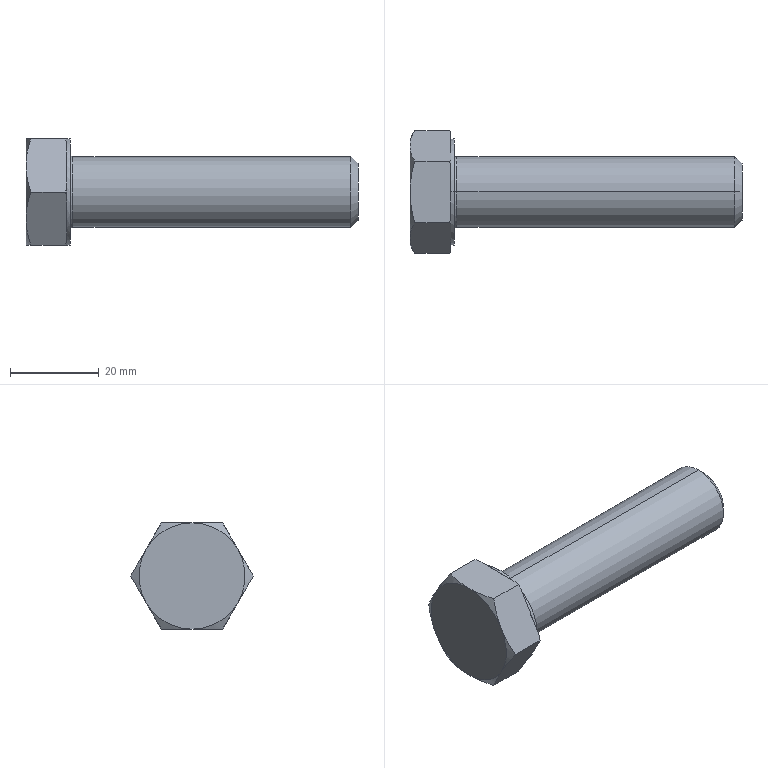Part | SolidWorks | features RevCut 4, Chamfer 1, Extrusion 1, Fillet 1, LPattern 1, Revolution 1 | 1 solid | 35 faces | box 75 x 27.713 x 24 mm | volume 17949 mm3 | plane 15 | cone 14 | cylinder 4 | torus 2 | commonest cylinder face diameters 16 x2 24 x2
STEP:
#1=CARTESIAN_POINT('',(10.6,0.,8.));
#2=VERTEX_POINT('',#1);
#3=CARTESIAN_POINT('',(10.6,0.,-8.));
#4=VERTEX_POINT('',#3);
#5=CARTESIAN_POINT('',(10.6,0.,0.));
#6=DIRECTION('',(1.,0.,0.));
#7=DIRECTION('',(0.,0.,-1.));
#8=AXIS2_PLACEMENT_3D('',#5,#6,#7);
#9=CIRCLE('',#8,8.);
#10=EDGE_CURVE('',#2,#4,#9,.T.);
#11=ORIENTED_EDGE('',*,*,#10,.F.);
#12=CARTESIAN_POINT('',(10.,0.,8.6));
#13=VERTEX_POINT('',#12);
#14=CARTESIAN_POINT('',(10.6,0.,8.6));
#15=DIRECTION('',(0.,1.,0.));
#16=DIRECTION('',(0.,0.,1.));
#17=AXIS2_PLACEMENT_3D('',#14,#15,#16);
#18=CIRCLE('',#17,0.6);
#19=EDGE_CURVE('',#2,#13,#18,.T.);
#20=ORIENTED_EDGE('',*,*,#19,.T.);
#21=CARTESIAN_POINT('',(10.,0.,-8.6));
#22=VERTEX_POINT('',#21);
#23=CARTESIAN_POINT('',(10.,0.,0.));
#24=DIRECTION('',(-1.,0.,0.));
#25=DIRECTION('',(0.,0.,-1.));
#26=AXIS2_PLACEMENT_3D('',#23,#24,#25);
#27=CIRCLE('',#26,8.6);
#28=EDGE_CURVE('',#22,#13,#27,.T.);
#29=ORIENTED_EDGE('',*,*,#28,.F.);
#30=CARTESIAN_POINT('',(10.6,0.,-8.6));
#31=DIRECTION('',(0.,-1.,0.));
#32=DIRECTION('',(0.,0.,-1.));
#33=AXIS2_PLACEMENT_3D('',#30,#31,#32);
#34=CIRCLE('',#33,0.6);
#35=EDGE_CURVE('',#4,#22,#34,.T.);
#36=ORIENTED_EDGE('',*,*,#35,.F.);
#37=EDGE_LOOP('',(#11,#20,#29,#36));
#38=FACE_OUTER_BOUND('',#37,.T.);
#39=CARTESIAN_POINT('',(10.6,0.,0.));
#40=DIRECTION('',(1.,0.,0.));
#41=DIRECTION('',(0.,0.,-1.));
#42=AXIS2_PLACEMENT_3D('',#39,#40,#41);
#43=TOROIDAL_SURFACE('',#42,8.6,0.6);
#44=ADVANCED_FACE('',(#38),#43,.F.);
#45=CARTESIAN_POINT('',(75.,0.,-6.4));
#46=VERTEX_POINT('',#45);
#47=CARTESIAN_POINT('',(75.,0.,6.4));
#48=VERTEX_POINT('',#47);
#49=CARTESIAN_POINT('',(75.,0.,0.));
#50=DIRECTION('',(1.,0.,0.));
#51=DIRECTION('',(0.,0.,1.));
#52=AXIS2_PLACEMENT_3D('',#49,#50,#51);
#53=CIRCLE('',#52,6.4);
#54=EDGE_CURVE('',#46,#48,#53,.T.);
#55=ORIENTED_EDGE('',*,*,#54,.F.);
#56=CARTESIAN_POINT('',(73.4,0.,-8.));
#57=VERTEX_POINT('',#56);
#58=CARTESIAN_POINT('',(73.4,0.,-8.));
#59=DIRECTION('',(-0.7071,0.,-0.7071));
#60=VECTOR('',#59,1000.);
#61=LINE('',#58,#60);
#62=EDGE_CURVE('',#46,#57,#61,.T.);
#63=ORIENTED_EDGE('',*,*,#62,.T.);
#64=CARTESIAN_POINT('',(73.4,0.,8.));
#65=VERTEX_POINT('',#64);
#66=CARTESIAN_POINT('',(73.4,0.,0.));
#67=DIRECTION('',(-1.,0.,0.));
#68=DIRECTION('',(0.,0.,1.));
#69=AXIS2_PLACEMENT_3D('',#66,#67,#68);
#70=CIRCLE('',#69,8.);
#71=EDGE_CURVE('',#65,#57,#70,.T.);
#72=ORIENTED_EDGE('',*,*,#71,.F.);
#73=CARTESIAN_POINT('',(73.4,0.,8.));
#74=DIRECTION('',(-0.7071,0.,0.7071));
#75=VECTOR('',#74,1000.);
#76=LINE('',#73,#75);
#77=EDGE_CURVE('',#48,#65,#76,.T.);
#78=ORIENTED_EDGE('',*,*,#77,.F.);
#79=EDGE_LOOP('',(#55,#63,#72,#78));
#80=FACE_OUTER_BOUND('',#79,.T.);
#81=CARTESIAN_POINT('',(73.4,0.,0.));
#82=DIRECTION('',(-1.,0.,0.));
#83=DIRECTION('',(0.,0.,1.));
#84=AXIS2_PLACEMENT_3D('',#81,#82,#83);
#85=CONICAL_SURFACE('',#84,8.,0.7854);
#86=ADVANCED_FACE('',(#80),#85,.T.);
#87=ORIENTED_EDGE('',*,*,#71,.T.);
#88=CARTESIAN_POINT('',(0.,0.,-8.));
#89=DIRECTION('',(-1.,0.,0.));
#90=VECTOR('',#89,1000.);
#91=LINE('',#88,#90);
#92=EDGE_CURVE('',#57,#4,#91,.T.);
#93=ORIENTED_EDGE('',*,*,#92,.T.);
#94=CARTESIAN_POINT('',(10.6,0.,0.));
#95=DIRECTION('',(1.,0.,0.));
#96=DIRECTION('',(0.,0.,-1.));
#97=AXIS2_PLACEMENT_3D('',#94,#95,#96);
#98=CIRCLE('',#97,8.);
#99=EDGE_CURVE('',#4,#2,#98,.T.);
#100=ORIENTED_EDGE('',*,*,#99,.T.);
#101=CARTESIAN_POINT('',(0.,0.,8.));
#102=DIRECTION('',(-1.,0.,0.));
#103=VECTOR('',#102,1000.);
#104=LINE('',#101,#103);
#105=EDGE_CURVE('',#65,#2,#104,.T.);
#106=ORIENTED_EDGE('',*,*,#105,.F.);
#107=EDGE_LOOP('',(#87,#93,#100,#106));
#108=FACE_OUTER_BOUND('',#107,.T.);
#109=CARTESIAN_POINT('',(0.,0.,0.));
#110=DIRECTION('',(-1.,0.,0.));
#111=DIRECTION('',(0.,0.,1.));
#112=AXIS2_PLACEMENT_3D('',#109,#110,#111);
#113=CYLINDRICAL_SURFACE('',#112,8.);
#114=ADVANCED_FACE('',(#108),#113,.T.);
#115=CARTESIAN_POINT('',(10.,0.,-12.));
#116=VERTEX_POINT('',#115);
#117=CARTESIAN_POINT('',(10.,0.,12.));
#118=VERTEX_POINT('',#117);
#119=CARTESIAN_POINT('',(10.,0.,0.));
#120=DIRECTION('',(1.,0.,0.));
#121=DIRECTION('',(0.,0.,-1.));
#122=AXIS2_PLACEMENT_3D('',#119,#120,#121);
#123=CIRCLE('',#122,12.);
#124=EDGE_CURVE('',#116,#118,#123,.T.);
#125=ORIENTED_EDGE('',*,*,#124,.F.);
#126=CARTESIAN_POINT('',(9.2,0.,-12.));
#127=VERTEX_POINT('',#126);
#128=CARTESIAN_POINT('',(0.,0.,-12.));
#129=DIRECTION('',(-1.,0.,0.));
#130=VECTOR('',#129,1000.);
#131=LINE('',#128,#130);
#132=EDGE_CURVE('',#116,#127,#131,.T.);
#133=ORIENTED_EDGE('',*,*,#132,.T.);
#134=CARTESIAN_POINT('',(9.2,10.392,-6.));
#135=VERTEX_POINT('',#134);
#136=CARTESIAN_POINT('',(9.2,0.,0.));
#137=DIRECTION('',(-1.,0.,0.));
#138=DIRECTION('',(0.,0.,1.));
#139=AXIS2_PLACEMENT_3D('',#136,#137,#138);
#140=CIRCLE('',#139,12.);
#141=EDGE_CURVE('',#135,#127,#140,.T.);
#142=ORIENTED_EDGE('',*,*,#141,.F.);
#143=CARTESIAN_POINT('',(9.2,10.392,6.));
#144=VERTEX_POINT('',#143);
#145=CARTESIAN_POINT('',(9.2,0.,0.));
#146=DIRECTION('',(-1.,0.,0.));
#147=DIRECTION('',(0.,0.,1.));
#148=AXIS2_PLACEMENT_3D('',#145,#146,#147);
#149=CIRCLE('',#148,12.);
#150=EDGE_CURVE('',#144,#135,#149,.T.);
#151=ORIENTED_EDGE('',*,*,#150,.F.);
#152=CARTESIAN_POINT('',(9.2,0.,12.));
#153=VERTEX_POINT('',#152);
#154=CARTESIAN_POINT('',(9.2,0.,0.));
#155=DIRECTION('',(-1.,0.,0.));
#156=DIRECTION('',(0.,0.,1.));
#157=AXIS2_PLACEMENT_3D('',#154,#155,#156);
#158=CIRCLE('',#157,12.);
#159=EDGE_CURVE('',#153,#144,#158,.T.);
#160=ORIENTED_EDGE('',*,*,#159,.F.);
#161=CARTESIAN_POINT('',(0.,0.,12.));
#162=DIRECTION('',(-1.,0.,0.));
#163=VECTOR('',#162,1000.);
#164=LINE('',#161,#163);
#165=EDGE_CURVE('',#118,#153,#164,.T.);
#166=ORIENTED_EDGE('',*,*,#165,.F.);
#167=EDGE_LOOP('',(#125,#133,#142,#151,#160,#166));
#168=FACE_OUTER_BOUND('',#167,.T.);
#169=CARTESIAN_POINT('',(0.,0.,0.));
#170=DIRECTION('',(-1.,0.,0.));
#171=DIRECTION('',(0.,0.,1.));
#172=AXIS2_PLACEMENT_3D('',#169,#170,#171);
#173=CYLINDRICAL_SURFACE('',#172,12.);
#174=ADVANCED_FACE('',(#168),#173,.T.);
#175=CARTESIAN_POINT('',(9.2,7.427,-11.136));
#176=VERTEX_POINT('',#175);
#177=CARTESIAN_POINT('',(9.2,6.928,-12.));
#178=DIRECTION('',(0.,0.5,0.866));
#179=VECTOR('',#178,1000.);
#180=LINE('',#177,#179);
#181=EDGE_CURVE('',#176,#135,#180,.T.);
#182=ORIENTED_EDGE('',*,*,#181,.F.);
#183=CARTESIAN_POINT('',(8.928,6.928,-12.));
#184=VERTEX_POINT('',#183);
#185=CARTESIAN_POINT('',(8.928,6.928,-12.));
#186=CARTESIAN_POINT('',(9.024,7.094,-11.713));
#187=CARTESIAN_POINT('',(9.115,7.26,-11.425));
#188=CARTESIAN_POINT('',(9.2,7.427,-11.136));
#189=B_SPLINE_CURVE_WITH_KNOTS('',3,(#185,#186,#187,#188),.UNSPECIFIED.,.F.,.F.,(4,4),(0.000000238,0.001026),.UNSPECIFIED.);
#190=EDGE_CURVE('',#184,#176,#189,.T.);
#191=ORIENTED_EDGE('',*,*,#190,.F.);
#192=CARTESIAN_POINT('',(1.072,6.928,-12.));
#193=VERTEX_POINT('',#192);
#194=CARTESIAN_POINT('',(10.,6.928,-12.));
#195=DIRECTION('',(-1.,0.,0.));
#196=VECTOR('',#195,1000.);
#197=LINE('',#194,#196);
#198=EDGE_CURVE('',#184,#193,#197,.T.);
#199=ORIENTED_EDGE('',*,*,#198,.T.);
#200=CARTESIAN_POINT('',(0.,10.392,-6.));
#201=VERTEX_POINT('',#200);
#202=CARTESIAN_POINT('',(0.,10.392,-6.));
#203=CARTESIAN_POINT('',(0.,10.098,-6.509));
#204=CARTESIAN_POINT('',(0.02533,9.803,-7.021));
#205=CARTESIAN_POINT('',(0.1234,9.219,-8.033));
#206=CARTESIAN_POINT('',(0.196,8.929,-8.535));
#207=CARTESIAN_POINT('',(0.476,8.063,-10.034));
#208=CARTESIAN_POINT('',(0.7454,7.493,-11.021));
#209=CARTESIAN_POINT('',(1.072,6.928,-12.));
#210=B_SPLINE_CURVE_WITH_KNOTS('',3,(#202,#203,#204,#205,#206,#207,#208,#209),.UNSPECIFIED.,.F.,.F.,(4,2,2,4),(0.00701,0.008756,0.0105,0.01399),.UNSPECIFIED.);
#211=EDGE_CURVE('',#201,#193,#210,.T.);
#212=ORIENTED_EDGE('',*,*,#211,.F.);
#213=CARTESIAN_POINT('',(1.072,13.856,0.));
#214=VERTEX_POINT('',#213);
#215=CARTESIAN_POINT('',(1.072,13.856,0.));
#216=CARTESIAN_POINT('',(0.7446,13.29,-0.9815));
#217=CARTESIAN_POINT('',(0.4751,12.719,-1.97));
#218=CARTESIAN_POINT('',(0.1021,11.565,-3.968));
#219=CARTESIAN_POINT('',(0.,10.982,-4.978));
#220=CARTESIAN_POINT('',(0.,10.392,-6.));
#221=B_SPLINE_CURVE_WITH_KNOTS('',3,(#215,#216,#217,#218,#219,#220),.UNSPECIFIED.,.F.,.F.,(4,2,4),(0.000000238,0.003505,0.00701),.UNSPECIFIED.);
#222=EDGE_CURVE('',#214,#201,#221,.T.);
#223=ORIENTED_EDGE('',*,*,#222,.F.);
#224=CARTESIAN_POINT('',(8.928,13.856,0.));
#225=VERTEX_POINT('',#224);
#226=CARTESIAN_POINT('',(10.,13.856,0.));
#227=DIRECTION('',(-1.,0.,0.));
#228=VECTOR('',#227,1000.);
#229=LINE('',#226,#228);
#230=EDGE_CURVE('',#225,#214,#229,.T.);
#231=ORIENTED_EDGE('',*,*,#230,.F.);
#232=CARTESIAN_POINT('',(9.2,13.358,-0.8637));
#233=VERTEX_POINT('',#232);
#234=CARTESIAN_POINT('',(9.2,13.358,-0.8637));
#235=CARTESIAN_POINT('',(9.115,13.524,-0.575));
#236=CARTESIAN_POINT('',(9.024,13.691,-0.2872));
#237=CARTESIAN_POINT('',(8.928,13.856,0.));
#238=B_SPLINE_CURVE_WITH_KNOTS('',3,(#234,#235,#236,#237),.UNSPECIFIED.,.F.,.F.,(4,4),(0.01297,0.01399),.UNSPECIFIED.);
#239=EDGE_CURVE('',#233,#225,#238,.T.);
#240=ORIENTED_EDGE('',*,*,#239,.F.);
#241=CARTESIAN_POINT('',(9.2,6.928,-12.));
#242=DIRECTION('',(0.,0.5,0.866));
#243=VECTOR('',#242,1000.);
#244=LINE('',#241,#243);
#245=EDGE_CURVE('',#135,#233,#244,.T.);
#246=ORIENTED_EDGE('',*,*,#245,.F.);
#247=EDGE_LOOP('',(#182,#191,#199,#212,#223,#231,#240,#246));
#248=FACE_OUTER_BOUND('',#247,.T.);
#249=CARTESIAN_POINT('',(10.,6.928,-12.));
#250=DIRECTION('',(0.,-0.866,0.5));
#251=DIRECTION('',(0.,-0.5,-0.866));
#252=AXIS2_PLACEMENT_3D('',#249,#250,#251);
#253=PLANE('',#252);
#254=ADVANCED_FACE('',(#248),#253,.F.);
#255=CARTESIAN_POINT('',(9.2,13.358,0.8637));
#256=VERTEX_POINT('',#255);
#257=CARTESIAN_POINT('',(9.2,13.856,0.));
#258=DIRECTION('',(0.,-0.5,0.866));
#259=VECTOR('',#258,1000.);
#260=LINE('',#257,#259);
#261=EDGE_CURVE('',#256,#144,#260,.T.);
#262=ORIENTED_EDGE('',*,*,#261,.F.);
#263=CARTESIAN_POINT('',(8.928,13.856,0.));
#264=CARTESIAN_POINT('',(9.024,13.691,0.2873));
#265=CARTESIAN_POINT('',(9.115,13.524,0.5751));
#266=CARTESIAN_POINT('',(9.2,13.358,0.8637));
#267=B_SPLINE_CURVE_WITH_KNOTS('',3,(#263,#264,#265,#266),.UNSPECIFIED.,.F.,.F.,(4,4),(0.000000238,0.001026),.UNSPECIFIED.);
#268=EDGE_CURVE('',#225,#256,#267,.T.);
#269=ORIENTED_EDGE('',*,*,#268,.F.);
#270=ORIENTED_EDGE('',*,*,#230,.T.);
#271=CARTESIAN_POINT('',(0.,10.392,6.));
#272=VERTEX_POINT('',#271);
#273=CARTESIAN_POINT('',(0.,10.392,6.));
#274=CARTESIAN_POINT('',(0.,10.686,5.491));
#275=CARTESIAN_POINT('',(0.02533,10.982,4.979));
#276=CARTESIAN_POINT('',(0.1234,11.566,3.967));
#277=CARTESIAN_POINT('',(0.196,11.856,3.465));
#278=CARTESIAN_POINT('',(0.476,12.721,1.966));
#279=CARTESIAN_POINT('',(0.7454,13.291,0.9791));
#280=CARTESIAN_POINT('',(1.072,13.856,0.));
#281=B_SPLINE_CURVE_WITH_KNOTS('',3,(#273,#274,#275,#276,#277,#278,#279,#280),.UNSPECIFIED.,.F.,.F.,(4,2,2,4),(0.00701,0.008756,0.0105,0.01399),.UNSPECIFIED.);
#282=EDGE_CURVE('',#272,#214,#281,.T.);
#283=ORIENTED_EDGE('',*,*,#282,.F.);
#284=CARTESIAN_POINT('',(1.072,6.928,12.));
#285=VERTEX_POINT('',#284);
#286=CARTESIAN_POINT('',(1.072,6.928,12.));
#287=CARTESIAN_POINT('',(0.7446,7.495,11.018));
#288=CARTESIAN_POINT('',(0.4751,8.066,10.03));
#289=CARTESIAN_POINT('',(0.1021,9.219,8.032));
#290=CARTESIAN_POINT('',(0.,9.802,7.022));
#291=CARTESIAN_POINT('',(0.,10.392,6.));
#292=B_SPLINE_CURVE_WITH_KNOTS('',3,(#286,#287,#288,#289,#290,#291),.UNSPECIFIED.,.F.,.F.,(4,2,4),(0.000000238,0.003505,0.00701),.UNSPECIFIED.);
#293=EDGE_CURVE('',#285,#272,#292,.T.);
#294=ORIENTED_EDGE('',*,*,#293,.F.);
#295=CARTESIAN_POINT('',(8.928,6.928,12.));
#296=VERTEX_POINT('',#295);
#297=CARTESIAN_POINT('',(10.,6.928,12.));
#298=DIRECTION('',(-1.,0.,0.));
#299=VECTOR('',#298,1000.);
#300=LINE('',#297,#299);
#301=EDGE_CURVE('',#296,#285,#300,.T.);
#302=ORIENTED_EDGE('',*,*,#301,.F.);
#303=CARTESIAN_POINT('',(9.2,7.427,11.136));
#304=VERTEX_POINT('',#303);
#305=CARTESIAN_POINT('',(9.2,7.427,11.136));
#306=CARTESIAN_POINT('',(9.115,7.26,11.425));
#307=CARTESIAN_POINT('',(9.024,7.094,11.713));
#308=CARTESIAN_POINT('',(8.928,6.928,12.));
#309=B_SPLINE_CURVE_WITH_KNOTS('',3,(#305,#306,#307,#308),.UNSPECIFIED.,.F.,.F.,(4,4),(0.01297,0.01399),.UNSPECIFIED.);
#310=EDGE_CURVE('',#304,#296,#309,.T.);
#311=ORIENTED_EDGE('',*,*,#310,.F.);
#312=CARTESIAN_POINT('',(9.2,13.856,0.));
#313=DIRECTION('',(0.,-0.5,0.866));
#314=VECTOR('',#313,1000.);
#315=LINE('',#312,#314);
#316=EDGE_CURVE('',#144,#304,#315,.T.);
#317=ORIENTED_EDGE('',*,*,#316,.F.);
#318=EDGE_LOOP('',(#262,#269,#270,#283,#294,#302,#311,#317));
#319=FACE_OUTER_BOUND('',#318,.T.);
#320=CARTESIAN_POINT('',(10.,13.856,0.));
#321=DIRECTION('',(0.,-0.866,-0.5));
#322=DIRECTION('',(0.,0.5,-0.866));
#323=AXIS2_PLACEMENT_3D('',#320,#321,#322);
#324=PLANE('',#323);
#325=ADVANCED_FACE('',(#319),#324,.F.);
#326=CARTESIAN_POINT('',(9.2,5.931,12.));
#327=VERTEX_POINT('',#326);
#328=CARTESIAN_POINT('',(9.2,6.928,12.));
#329=DIRECTION('',(0.,-1.,0.));
#330=VECTOR('',#329,1000.);
#331=LINE('',#328,#330);
#332=EDGE_CURVE('',#327,#153,#331,.T.);
#333=ORIENTED_EDGE('',*,*,#332,.F.);
#334=CARTESIAN_POINT('',(8.928,6.928,12.));
#335=CARTESIAN_POINT('',(9.024,6.597,12.));
#336=CARTESIAN_POINT('',(9.115,6.265,12.));
#337=CARTESIAN_POINT('',(9.2,5.931,12.));
#338=B_SPLINE_CURVE_WITH_KNOTS('',3,(#334,#335,#336,#337),.UNSPECIFIED.,.F.,.F.,(4,4),(0.03236,0.0334),.UNSPECIFIED.);
#339=EDGE_CURVE('',#296,#327,#338,.T.);
#340=ORIENTED_EDGE('',*,*,#339,.F.);
#341=ORIENTED_EDGE('',*,*,#301,.T.);
#342=CARTESIAN_POINT('',(0.,0.,12.));
#343=VERTEX_POINT('',#342);
#344=CARTESIAN_POINT('',(0.,0.,12.));
#345=CARTESIAN_POINT('',(0.,0.5865,12.));
#346=CARTESIAN_POINT('',(0.02506,1.176,12.));
#347=CARTESIAN_POINT('',(0.1242,2.355,12.));
#348=CARTESIAN_POINT('',(0.1975,2.939,12.));
#349=CARTESIAN_POINT('',(0.4791,4.673,12.));
#350=CARTESIAN_POINT('',(0.7483,5.808,12.));
#351=CARTESIAN_POINT('',(1.072,6.928,12.));
#352=B_SPLINE_CURVE_WITH_KNOTS('',3,(#344,#345,#346,#347,#348,#349,#350,#351),.UNSPECIFIED.,.F.,.F.,(4,2,2,4),(0.01982,0.02158,0.02333,0.02684),.UNSPECIFIED.);
#353=EDGE_CURVE('',#343,#285,#352,.T.);
#354=ORIENTED_EDGE('',*,*,#353,.F.);
#355=CARTESIAN_POINT('',(1.072,-6.928,12.));
#356=VERTEX_POINT('',#355);
#357=CARTESIAN_POINT('',(1.072,-6.928,12.));
#358=CARTESIAN_POINT('',(0.7461,-5.8,12.));
#359=CARTESIAN_POINT('',(0.4736,-4.647,12.));
#360=CARTESIAN_POINT('',(0.1008,-2.335,12.));
#361=CARTESIAN_POINT('',(0.,-1.172,12.));
#362=CARTESIAN_POINT('',(0.,0.,12.));
#363=B_SPLINE_CURVE_WITH_KNOTS('',3,(#357,#358,#359,#360,#361,#362),.UNSPECIFIED.,.F.,.F.,(4,2,4),(0.01281,0.01632,0.01982),.UNSPECIFIED.);
#364=EDGE_CURVE('',#356,#343,#363,.T.);
#365=ORIENTED_EDGE('',*,*,#364,.F.);
#366=CARTESIAN_POINT('',(8.928,-6.928,12.));
#367=VERTEX_POINT('',#366);
#368=CARTESIAN_POINT('',(10.,-6.928,12.));
#369=DIRECTION('',(-1.,0.,0.));
#370=VECTOR('',#369,1000.);
#371=LINE('',#368,#370);
#372=EDGE_CURVE('',#367,#356,#371,.T.);
#373=ORIENTED_EDGE('',*,*,#372,.F.);
#374=CARTESIAN_POINT('',(9.2,-5.931,12.));
#375=VERTEX_POINT('',#374);
#376=CARTESIAN_POINT('',(9.2,-5.931,12.));
#377=CARTESIAN_POINT('',(9.114,-6.265,12.));
#378=CARTESIAN_POINT('',(9.024,-6.598,12.));
#379=CARTESIAN_POINT('',(8.928,-6.928,12.));
#380=B_SPLINE_CURVE_WITH_KNOTS('',3,(#376,#377,#378,#379),.UNSPECIFIED.,.F.,.F.,(4,4),(0.04537,0.0464),.UNSPECIFIED.);
#381=EDGE_CURVE('',#375,#367,#380,.T.);
#382=ORIENTED_EDGE('',*,*,#381,.F.);
#383=CARTESIAN_POINT('',(9.2,6.928,12.));
#384=DIRECTION('',(0.,-1.,0.));
#385=VECTOR('',#384,1000.);
#386=LINE('',#383,#385);
#387=EDGE_CURVE('',#153,#375,#386,.T.);
#388=ORIENTED_EDGE('',*,*,#387,.F.);
#389=EDGE_LOOP('',(#333,#340,#341,#354,#365,#373,#382,#388));
#390=FACE_OUTER_BOUND('',#389,.T.);
#391=CARTESIAN_POINT('',(10.,6.928,12.));
#392=DIRECTION('',(0.,0.,-1.));
#393=DIRECTION('',(0.,1.,0.));
#394=AXIS2_PLACEMENT_3D('',#391,#392,#393);
#395=PLANE('',#394);
#396=ADVANCED_FACE('',(#390),#395,.F.);
#397=CARTESIAN_POINT('',(9.2,-7.427,11.136));
#398=VERTEX_POINT('',#397);
#399=CARTESIAN_POINT('',(9.2,-10.392,6.));
#400=VERTEX_POINT('',#399);
#401=CARTESIAN_POINT('',(9.2,-13.856,0.));
#402=DIRECTION('',(0.,-0.5,-0.866));
#403=VECTOR('',#402,1000.);
#404=LINE('',#401,#403);
#405=EDGE_CURVE('',#398,#400,#404,.T.);
#406=ORIENTED_EDGE('',*,*,#405,.F.);
#407=CARTESIAN_POINT('',(8.928,-6.928,12.));
#408=CARTESIAN_POINT('',(9.024,-7.094,11.713));
#409=CARTESIAN_POINT('',(9.115,-7.26,11.425));
#410=CARTESIAN_POINT('',(9.2,-7.427,11.136));
#411=B_SPLINE_CURVE_WITH_KNOTS('',3,(#407,#408,#409,#410),.UNSPECIFIED.,.F.,.F.,(4,4),(0.000000238,0.001026),.UNSPECIFIED.);
#412=EDGE_CURVE('',#367,#398,#411,.T.);
#413=ORIENTED_EDGE('',*,*,#412,.F.);
#414=ORIENTED_EDGE('',*,*,#372,.T.);
#415=CARTESIAN_POINT('',(0.,-10.392,6.));
#416=VERTEX_POINT('',#415);
#417=CARTESIAN_POINT('',(0.,-10.392,6.));
#418=CARTESIAN_POINT('',(0.,-10.098,6.509));
#419=CARTESIAN_POINT('',(0.02533,-9.803,7.021));
#420=CARTESIAN_POINT('',(0.1234,-9.219,8.033));
#421=CARTESIAN_POINT('',(0.196,-8.929,8.535));
#422=CARTESIAN_POINT('',(0.476,-8.063,10.034));
#423=CARTESIAN_POINT('',(0.7454,-7.493,11.021));
#424=CARTESIAN_POINT('',(1.072,-6.928,12.));
#425=B_SPLINE_CURVE_WITH_KNOTS('',3,(#417,#418,#419,#420,#421,#422,#423,#424),.UNSPECIFIED.,.F.,.F.,(4,2,2,4),(0.00701,0.008756,0.0105,0.01399),.UNSPECIFIED.);
#426=EDGE_CURVE('',#416,#356,#425,.T.);
#427=ORIENTED_EDGE('',*,*,#426,.F.);
#428=CARTESIAN_POINT('',(1.072,-13.856,0.));
#429=VERTEX_POINT('',#428);
#430=CARTESIAN_POINT('',(1.072,-13.856,0.));
#431=CARTESIAN_POINT('',(0.7446,-13.29,0.9815));
#432=CARTESIAN_POINT('',(0.4751,-12.719,1.97));
#433=CARTESIAN_POINT('',(0.1021,-11.565,3.968));
#434=CARTESIAN_POINT('',(0.,-10.982,4.978));
#435=CARTESIAN_POINT('',(0.,-10.392,6.));
#436=B_SPLINE_CURVE_WITH_KNOTS('',3,(#430,#431,#432,#433,#434,#435),.UNSPECIFIED.,.F.,.F.,(4,2,4),(0.000000238,0.003505,0.00701),.UNSPECIFIED.);
#437=EDGE_CURVE('',#429,#416,#436,.T.);
#438=ORIENTED_EDGE('',*,*,#437,.F.);
#439=CARTESIAN_POINT('',(8.928,-13.856,0.));
#440=VERTEX_POINT('',#439);
#441=CARTESIAN_POINT('',(10.,-13.856,0.));
#442=DIRECTION('',(-1.,0.,0.));
#443=VECTOR('',#442,1000.);
#444=LINE('',#441,#443);
#445=EDGE_CURVE('',#440,#429,#444,.T.);
#446=ORIENTED_EDGE('',*,*,#445,.F.);
#447=CARTESIAN_POINT('',(9.2,-13.358,0.8637));
#448=VERTEX_POINT('',#447);
#449=CARTESIAN_POINT('',(9.2,-13.358,0.8637));
#450=CARTESIAN_POINT('',(9.115,-13.524,0.575));
#451=CARTESIAN_POINT('',(9.024,-13.691,0.2872));
#452=CARTESIAN_POINT('',(8.928,-13.856,0.));
#453=B_SPLINE_CURVE_WITH_KNOTS('',3,(#449,#450,#451,#452),.UNSPECIFIED.,.F.,.F.,(4,4),(0.01297,0.01399),.UNSPECIFIED.);
#454=EDGE_CURVE('',#448,#440,#453,.T.);
#455=ORIENTED_EDGE('',*,*,#454,.F.);
#456=CARTESIAN_POINT('',(9.2,-13.856,0.));
#457=DIRECTION('',(0.,-0.5,-0.866));
#458=VECTOR('',#457,1000.);
#459=LINE('',#456,#458);
#460=EDGE_CURVE('',#400,#448,#459,.T.);
#461=ORIENTED_EDGE('',*,*,#460,.F.);
#462=EDGE_LOOP('',(#406,#413,#414,#427,#438,#446,#455,#461));
#463=FACE_OUTER_BOUND('',#462,.T.);
#464=CARTESIAN_POINT('',(10.,-13.856,0.));
#465=DIRECTION('',(0.,0.866,-0.5));
#466=DIRECTION('',(0.,0.5,0.866));
#467=AXIS2_PLACEMENT_3D('',#464,#465,#466);
#468=PLANE('',#467);
#469=ADVANCED_FACE('',(#463),#468,.F.);
#470=CARTESIAN_POINT('',(9.2,-13.358,-0.8637));
#471=VERTEX_POINT('',#470);
#472=CARTESIAN_POINT('',(9.2,-10.392,-6.));
#473=VERTEX_POINT('',#472);
#474=CARTESIAN_POINT('',(9.2,-6.928,-12.));
#475=DIRECTION('',(0.,0.5,-0.866));
#476=VECTOR('',#475,1000.);
#477=LINE('',#474,#476);
#478=EDGE_CURVE('',#471,#473,#477,.T.);
#479=ORIENTED_EDGE('',*,*,#478,.F.);
#480=CARTESIAN_POINT('',(8.928,-13.856,0.));
#481=CARTESIAN_POINT('',(9.024,-13.691,-0.2873));
#482=CARTESIAN_POINT('',(9.115,-13.524,-0.5751));
#483=CARTESIAN_POINT('',(9.2,-13.358,-0.8637));
#484=B_SPLINE_CURVE_WITH_KNOTS('',3,(#480,#481,#482,#483),.UNSPECIFIED.,.F.,.F.,(4,4),(0.000000238,0.001026),.UNSPECIFIED.);
#485=EDGE_CURVE('',#440,#471,#484,.T.);
#486=ORIENTED_EDGE('',*,*,#485,.F.);
#487=ORIENTED_EDGE('',*,*,#445,.T.);
#488=CARTESIAN_POINT('',(0.,-10.392,-6.));
#489=VERTEX_POINT('',#488);
#490=CARTESIAN_POINT('',(0.,-10.392,-6.));
#491=CARTESIAN_POINT('',(0.,-10.686,-5.491));
#492=CARTESIAN_POINT('',(0.02533,-10.982,-4.979));
#493=CARTESIAN_POINT('',(0.1234,-11.566,-3.967));
#494=CARTESIAN_POINT('',(0.196,-11.856,-3.465));
#495=CARTESIAN_POINT('',(0.476,-12.721,-1.966));
#496=CARTESIAN_POINT('',(0.7454,-13.291,-0.9791));
#497=CARTESIAN_POINT('',(1.072,-13.856,0.));
#498=B_SPLINE_CURVE_WITH_KNOTS('',3,(#490,#491,#492,#493,#494,#495,#496,#497),.UNSPECIFIED.,.F.,.F.,(4,2,2,4),(0.00701,0.008756,0.0105,0.01399),.UNSPECIFIED.);
#499=EDGE_CURVE('',#489,#429,#498,.T.);
#500=ORIENTED_EDGE('',*,*,#499,.F.);
#501=CARTESIAN_POINT('',(1.072,-6.928,-12.));
#502=VERTEX_POINT('',#501);
#503=CARTESIAN_POINT('',(1.072,-6.928,-12.));
#504=CARTESIAN_POINT('',(0.7446,-7.495,-11.018));
#505=CARTESIAN_POINT('',(0.4751,-8.066,-10.03));
#506=CARTESIAN_POINT('',(0.1021,-9.219,-8.032));
#507=CARTESIAN_POINT('',(0.,-9.802,-7.022));
#508=CARTESIAN_POINT('',(0.,-10.392,-6.));
#509=B_SPLINE_CURVE_WITH_KNOTS('',3,(#503,#504,#505,#506,#507,#508),.UNSPECIFIED.,.F.,.F.,(4,2,4),(0.000000238,0.003505,0.00701),.UNSPECIFIED.);
#510=EDGE_CURVE('',#502,#489,#509,.T.);
#511=ORIENTED_EDGE('',*,*,#510,.F.);
#512=CARTESIAN_POINT('',(8.928,-6.928,-12.));
#513=VERTEX_POINT('',#512);
#514=CARTESIAN_POINT('',(10.,-6.928,-12.));
#515=DIRECTION('',(-1.,0.,0.));
#516=VECTOR('',#515,1000.);
#517=LINE('',#514,#516);
#518=EDGE_CURVE('',#513,#502,#517,.T.);
#519=ORIENTED_EDGE('',*,*,#518,.F.);
#520=CARTESIAN_POINT('',(9.2,-7.427,-11.136));
#521=VERTEX_POINT('',#520);
#522=CARTESIAN_POINT('',(9.2,-7.427,-11.136));
#523=CARTESIAN_POINT('',(9.115,-7.26,-11.425));
#524=CARTESIAN_POINT('',(9.024,-7.094,-11.713));
#525=CARTESIAN_POINT('',(8.928,-6.928,-12.));
#526=B_SPLINE_CURVE_WITH_KNOTS('',3,(#522,#523,#524,#525),.UNSPECIFIED.,.F.,.F.,(4,4),(0.01297,0.01399),.UNSPECIFIED.);
#527=EDGE_CURVE('',#521,#513,#526,.T.);
#528=ORIENTED_EDGE('',*,*,#527,.F.);
#529=CARTESIAN_POINT('',(9.2,-6.928,-12.));
#530=DIRECTION('',(0.,0.5,-0.866));
#531=VECTOR('',#530,1000.);
#532=LINE('',#529,#531);
#533=EDGE_CURVE('',#473,#521,#532,.T.);
#534=ORIENTED_EDGE('',*,*,#533,.F.);
#535=EDGE_LOOP('',(#479,#486,#487,#500,#511,#519,#528,#534));
#536=FACE_OUTER_BOUND('',#535,.T.);
#537=CARTESIAN_POINT('',(10.,-6.928,-12.));
#538=DIRECTION('',(0.,0.866,0.5));
#539=DIRECTION('',(0.,-0.5,0.866));
#540=AXIS2_PLACEMENT_3D('',#537,#538,#539);
#541=PLANE('',#540);
#542=ADVANCED_FACE('',(#536),#541,.F.);
#543=CARTESIAN_POINT('',(9.2,-5.931,-12.));
#544=VERTEX_POINT('',#543);
#545=CARTESIAN_POINT('',(9.2,6.928,-12.));
#546=DIRECTION('',(0.,1.,0.));
#547=VECTOR('',#546,1000.);
#548=LINE('',#545,#547);
#549=EDGE_CURVE('',#544,#127,#548,.T.);
#550=ORIENTED_EDGE('',*,*,#549,.F.);
#551=CARTESIAN_POINT('',(8.928,-6.928,-12.));
#552=CARTESIAN_POINT('',(9.024,-6.598,-12.));
#553=CARTESIAN_POINT('',(9.114,-6.265,-12.));
#554=CARTESIAN_POINT('',(9.2,-5.931,-12.));
#555=B_SPLINE_CURVE_WITH_KNOTS('',3,(#551,#552,#553,#554),.UNSPECIFIED.,.F.,.F.,(4,4),(0.01281,0.01384),.UNSPECIFIED.);
#556=EDGE_CURVE('',#513,#544,#555,.T.);
#557=ORIENTED_EDGE('',*,*,#556,.F.);
#558=ORIENTED_EDGE('',*,*,#518,.T.);
#559=CARTESIAN_POINT('',(0.,0.,-12.));
#560=VERTEX_POINT('',#559);
#561=CARTESIAN_POINT('',(0.,0.,-12.));
#562=CARTESIAN_POINT('',(0.,-1.172,-12.));
#563=CARTESIAN_POINT('',(0.1008,-2.335,-12.));
#564=CARTESIAN_POINT('',(0.4736,-4.647,-12.));
#565=CARTESIAN_POINT('',(0.7461,-5.8,-12.));
#566=CARTESIAN_POINT('',(1.072,-6.928,-12.));
#567=B_SPLINE_CURVE_WITH_KNOTS('',3,(#561,#562,#563,#564,#565,#566),.UNSPECIFIED.,.F.,.F.,(4,2,4),(0.03938,0.04289,0.0464),.UNSPECIFIED.);
#568=EDGE_CURVE('',#560,#502,#567,.T.);
#569=ORIENTED_EDGE('',*,*,#568,.F.);
#570=CARTESIAN_POINT('',(1.072,6.928,-12.));
#571=CARTESIAN_POINT('',(0.7483,5.808,-12.));
#572=CARTESIAN_POINT('',(0.4791,4.673,-12.));
#573=CARTESIAN_POINT('',(0.1975,2.939,-12.));
#574=CARTESIAN_POINT('',(0.1242,2.355,-12.));
#575=CARTESIAN_POINT('',(0.02506,1.176,-12.));
#576=CARTESIAN_POINT('',(0.,0.5865,-12.));
#577=CARTESIAN_POINT('',(0.,0.,-12.));
#578=B_SPLINE_CURVE_WITH_KNOTS('',3,(#570,#571,#572,#573,#574,#575,#576,#577),.UNSPECIFIED.,.F.,.F.,(4,2,2,4),(0.03236,0.03587,0.03763,0.03938),.UNSPECIFIED.);
#579=EDGE_CURVE('',#193,#560,#578,.T.);
#580=ORIENTED_EDGE('',*,*,#579,.F.);
#581=ORIENTED_EDGE('',*,*,#198,.F.);
#582=CARTESIAN_POINT('',(9.2,5.931,-12.));
#583=VERTEX_POINT('',#582);
#584=CARTESIAN_POINT('',(9.2,5.931,-12.));
#585=CARTESIAN_POINT('',(9.115,6.265,-12.));
#586=CARTESIAN_POINT('',(9.024,6.597,-12.));
#587=CARTESIAN_POINT('',(8.928,6.928,-12.));
#588=B_SPLINE_CURVE_WITH_KNOTS('',3,(#584,#585,#586,#587),.UNSPECIFIED.,.F.,.F.,(4,4),(0.0258,0.02684),.UNSPECIFIED.);
#589=EDGE_CURVE('',#583,#184,#588,.T.);
#590=ORIENTED_EDGE('',*,*,#589,.F.);
#591=CARTESIAN_POINT('',(9.2,6.928,-12.));
#592=DIRECTION('',(0.,1.,0.));
#593=VECTOR('',#592,1000.);
#594=LINE('',#591,#593);
#595=EDGE_CURVE('',#127,#583,#594,.T.);
#596=ORIENTED_EDGE('',*,*,#595,.F.);
#597=EDGE_LOOP('',(#550,#557,#558,#569,#580,#581,#590,#596));
#598=FACE_OUTER_BOUND('',#597,.T.);
#599=CARTESIAN_POINT('',(10.,6.928,-12.));
#600=DIRECTION('',(0.,0.,1.));
#601=DIRECTION('',(0.,-1.,0.));
#602=AXIS2_PLACEMENT_3D('',#599,#600,#601);
#603=PLANE('',#602);
#604=ADVANCED_FACE('',(#598),#603,.F.);
#605=ORIENTED_EDGE('',*,*,#556,.T.);
#606=CARTESIAN_POINT('',(9.2,0.,0.));
#607=DIRECTION('',(-1.,0.,0.));
#608=DIRECTION('',(0.,0.,-1.));
#609=AXIS2_PLACEMENT_3D('',#606,#607,#608);
#610=CIRCLE('',#609,13.386);
#611=EDGE_CURVE('',#544,#521,#610,.T.);
#612=ORIENTED_EDGE('',*,*,#611,.T.);
#613=ORIENTED_EDGE('',*,*,#527,.T.);
#614=EDGE_LOOP('',(#605,#612,#613));
#615=FACE_OUTER_BOUND('',#614,.T.);
#616=CARTESIAN_POINT('',(6.041,0.,0.));
#617=DIRECTION('',(-1.,0.,0.));
#618=DIRECTION('',(0.,0.,1.));
#619=AXIS2_PLACEMENT_3D('',#616,#617,#618);
#620=CONICAL_SURFACE('',#619,18.856,1.047);
#621=ADVANCED_FACE('',(#615),#620,.T.);
#622=ORIENTED_EDGE('',*,*,#485,.T.);
#623=CARTESIAN_POINT('',(9.2,0.,0.));
#624=DIRECTION('',(-1.,0.,0.));
#625=DIRECTION('',(0.,0.,-1.));
#626=AXIS2_PLACEMENT_3D('',#623,#624,#625);
#627=CIRCLE('',#626,13.386);
#628=EDGE_CURVE('',#471,#448,#627,.T.);
#629=ORIENTED_EDGE('',*,*,#628,.T.);
#630=ORIENTED_EDGE('',*,*,#454,.T.);
#631=EDGE_LOOP('',(#622,#629,#630));
#632=FACE_OUTER_BOUND('',#631,.T.);
#633=CARTESIAN_POINT('',(6.041,0.,0.));
#634=DIRECTION('',(-1.,0.,0.));
#635=DIRECTION('',(0.,0.,1.));
#636=AXIS2_PLACEMENT_3D('',#633,#634,#635);
#637=CONICAL_SURFACE('',#636,18.856,1.047);
#638=ADVANCED_FACE('',(#632),#637,.T.);
#639=ORIENTED_EDGE('',*,*,#412,.T.);
#640=CARTESIAN_POINT('',(9.2,0.,0.));
#641=DIRECTION('',(-1.,0.,0.));
#642=DIRECTION('',(0.,0.,-1.));
#643=AXIS2_PLACEMENT_3D('',#640,#641,#642);
#644=CIRCLE('',#643,13.386);
#645=EDGE_CURVE('',#398,#375,#644,.T.);
#646=ORIENTED_EDGE('',*,*,#645,.T.);
#647=ORIENTED_EDGE('',*,*,#381,.T.);
#648=EDGE_LOOP('',(#639,#646,#647));
#649=FACE_OUTER_BOUND('',#648,.T.);
#650=CARTESIAN_POINT('',(6.041,0.,0.));
#651=DIRECTION('',(-1.,0.,0.));
#652=DIRECTION('',(0.,0.,1.));
#653=AXIS2_PLACEMENT_3D('',#650,#651,#652);
#654=CONICAL_SURFACE('',#653,18.856,1.047);
#655=ADVANCED_FACE('',(#649),#654,.T.);
#656=ORIENTED_EDGE('',*,*,#339,.T.);
#657=CARTESIAN_POINT('',(9.2,0.,0.));
#658=DIRECTION('',(-1.,0.,0.));
#659=DIRECTION('',(0.,0.,-1.));
#660=AXIS2_PLACEMENT_3D('',#657,#658,#659);
#661=CIRCLE('',#660,13.386);
#662=EDGE_CURVE('',#327,#304,#661,.T.);
#663=ORIENTED_EDGE('',*,*,#662,.T.);
#664=ORIENTED_EDGE('',*,*,#310,.T.);
#665=EDGE_LOOP('',(#656,#663,#664));
#666=FACE_OUTER_BOUND('',#665,.T.);
#667=CARTESIAN_POINT('',(6.041,0.,0.));
#668=DIRECTION('',(-1.,0.,0.));
#669=DIRECTION('',(0.,0.,1.));
#670=AXIS2_PLACEMENT_3D('',#667,#668,#669);
#671=CONICAL_SURFACE('',#670,18.856,1.047);
#672=ADVANCED_FACE('',(#666),#671,.T.);
#673=ORIENTED_EDGE('',*,*,#268,.T.);
#674=CARTESIAN_POINT('',(9.2,0.,0.));
#675=DIRECTION('',(-1.,0.,0.));
#676=DIRECTION('',(0.,0.,-1.));
#677=AXIS2_PLACEMENT_3D('',#674,#675,#676);
#678=CIRCLE('',#677,13.386);
#679=EDGE_CURVE('',#256,#233,#678,.T.);
#680=ORIENTED_EDGE('',*,*,#679,.T.);
#681=ORIENTED_EDGE('',*,*,#239,.T.);
#682=EDGE_LOOP('',(#673,#680,#681));
#683=FACE_OUTER_BOUND('',#682,.T.);
#684=CARTESIAN_POINT('',(6.041,0.,0.));
#685=DIRECTION('',(-1.,0.,0.));
#686=DIRECTION('',(0.,0.,1.));
#687=AXIS2_PLACEMENT_3D('',#684,#685,#686);
#688=CONICAL_SURFACE('',#687,18.856,1.047);
#689=ADVANCED_FACE('',(#683),#688,.T.);
#690=ORIENTED_EDGE('',*,*,#190,.T.);
#691=CARTESIAN_POINT('',(9.2,0.,0.));
#692=DIRECTION('',(-1.,0.,0.));
#693=DIRECTION('',(0.,0.,-1.));
#694=AXIS2_PLACEMENT_3D('',#691,#692,#693);
#695=CIRCLE('',#694,13.386);
#696=EDGE_CURVE('',#176,#583,#695,.T.);
#697=ORIENTED_EDGE('',*,*,#696,.T.);
#698=ORIENTED_EDGE('',*,*,#589,.T.);
#699=EDGE_LOOP('',(#690,#697,#698));
#700=FACE_OUTER_BOUND('',#699,.T.);
#701=CARTESIAN_POINT('',(6.041,0.,0.));
#702=DIRECTION('',(-1.,0.,0.));
#703=DIRECTION('',(0.,0.,1.));
#704=AXIS2_PLACEMENT_3D('',#701,#702,#703);
#705=CONICAL_SURFACE('',#704,18.856,1.047);
#706=ADVANCED_FACE('',(#700),#705,.T.);
#707=ORIENTED_EDGE('',*,*,#510,.T.);
#708=CARTESIAN_POINT('',(0.,0.,0.));
#709=DIRECTION('',(1.,0.,0.));
#710=DIRECTION('',(0.,0.,-1.));
#711=AXIS2_PLACEMENT_3D('',#708,#709,#710);
#712=CIRCLE('',#711,12.);
#713=EDGE_CURVE('',#489,#560,#712,.T.);
#714=ORIENTED_EDGE('',*,*,#713,.T.);
#715=ORIENTED_EDGE('',*,*,#568,.T.);
#716=EDGE_LOOP('',(#707,#714,#715));
#717=FACE_OUTER_BOUND('',#716,.T.);
#718=CARTESIAN_POINT('',(0.,0.,0.));
#719=DIRECTION('',(1.,0.,0.));
#720=DIRECTION('',(0.,0.,-1.));
#721=AXIS2_PLACEMENT_3D('',#718,#719,#720);
#722=CONICAL_SURFACE('',#721,12.,1.047);
#723=ADVANCED_FACE('',(#717),#722,.T.);
#724=ORIENTED_EDGE('',*,*,#437,.T.);
#725=CARTESIAN_POINT('',(0.,0.,0.));
#726=DIRECTION('',(1.,0.,0.));
#727=DIRECTION('',(0.,0.,-1.));
#728=AXIS2_PLACEMENT_3D('',#725,#726,#727);
#729=CIRCLE('',#728,12.);
#730=EDGE_CURVE('',#416,#489,#729,.T.);
#731=ORIENTED_EDGE('',*,*,#730,.T.);
#732=ORIENTED_EDGE('',*,*,#499,.T.);
#733=EDGE_LOOP('',(#724,#731,#732));
#734=FACE_OUTER_BOUND('',#733,.T.);
#735=CARTESIAN_POINT('',(0.,0.,0.));
#736=DIRECTION('',(1.,0.,0.));
#737=DIRECTION('',(0.,0.,-1.));
#738=AXIS2_PLACEMENT_3D('',#735,#736,#737);
#739=CONICAL_SURFACE('',#738,12.,1.047);
#740=ADVANCED_FACE('',(#734),#739,.T.);
#741=ORIENTED_EDGE('',*,*,#364,.T.);
#742=CARTESIAN_POINT('',(0.,0.,0.));
#743=DIRECTION('',(1.,0.,0.));
#744=DIRECTION('',(0.,0.,-1.));
#745=AXIS2_PLACEMENT_3D('',#742,#743,#744);
#746=CIRCLE('',#745,12.);
#747=EDGE_CURVE('',#343,#416,#746,.T.);
#748=ORIENTED_EDGE('',*,*,#747,.T.);
#749=ORIENTED_EDGE('',*,*,#426,.T.);
#750=EDGE_LOOP('',(#741,#748,#749));
#751=FACE_OUTER_BOUND('',#750,.T.);
#752=CARTESIAN_POINT('',(0.,0.,0.));
#753=DIRECTION('',(1.,0.,0.));
#754=DIRECTION('',(0.,0.,-1.));
#755=AXIS2_PLACEMENT_3D('',#752,#753,#754);
#756=CONICAL_SURFACE('',#755,12.,1.047);
#757=ADVANCED_FACE('',(#751),#756,.T.);
#758=ORIENTED_EDGE('',*,*,#353,.T.);
#759=ORIENTED_EDGE('',*,*,#293,.T.);
#760=CARTESIAN_POINT('',(0.,0.,0.));
#761=DIRECTION('',(-1.,0.,0.));
#762=DIRECTION('',(0.,0.,1.));
#763=AXIS2_PLACEMENT_3D('',#760,#761,#762);
#764=CIRCLE('',#763,12.);
#765=EDGE_CURVE('',#343,#272,#764,.T.);
#766=ORIENTED_EDGE('',*,*,#765,.F.);
#767=EDGE_LOOP('',(#758,#759,#766));
#768=FACE_OUTER_BOUND('',#767,.T.);
#769=CARTESIAN_POINT('',(0.,0.,0.));
#770=DIRECTION('',(1.,0.,0.));
#771=DIRECTION('',(0.,0.,-1.));
#772=AXIS2_PLACEMENT_3D('',#769,#770,#771);
#773=CONICAL_SURFACE('',#772,12.,1.047);
#774=ADVANCED_FACE('',(#768),#773,.T.);
#775=ORIENTED_EDGE('',*,*,#282,.T.);
#776=ORIENTED_EDGE('',*,*,#222,.T.);
#777=CARTESIAN_POINT('',(0.,0.,0.));
#778=DIRECTION('',(1.,0.,0.));
#779=DIRECTION('',(0.,0.,-1.));
#780=AXIS2_PLACEMENT_3D('',#777,#778,#779);
#781=CIRCLE('',#780,12.);
#782=EDGE_CURVE('',#201,#272,#781,.T.);
#783=ORIENTED_EDGE('',*,*,#782,.T.);
#784=EDGE_LOOP('',(#775,#776,#783));
#785=FACE_OUTER_BOUND('',#784,.T.);
#786=CARTESIAN_POINT('',(0.,0.,0.));
#787=DIRECTION('',(1.,0.,0.));
#788=DIRECTION('',(0.,0.,-1.));
#789=AXIS2_PLACEMENT_3D('',#786,#787,#788);
#790=CONICAL_SURFACE('',#789,12.,1.047);
#791=ADVANCED_FACE('',(#785),#790,.T.);
#792=ORIENTED_EDGE('',*,*,#211,.T.);
#793=ORIENTED_EDGE('',*,*,#579,.T.);
#794=CARTESIAN_POINT('',(0.,0.,0.));
#795=DIRECTION('',(1.,0.,0.));
#796=DIRECTION('',(0.,0.,-1.));
#797=AXIS2_PLACEMENT_3D('',#794,#795,#796);
#798=CIRCLE('',#797,12.);
#799=EDGE_CURVE('',#560,#201,#798,.T.);
#800=ORIENTED_EDGE('',*,*,#799,.T.);
#801=EDGE_LOOP('',(#792,#793,#800));
#802=FACE_OUTER_BOUND('',#801,.T.);
#803=CARTESIAN_POINT('',(0.,0.,0.));
#804=DIRECTION('',(1.,0.,0.));
#805=DIRECTION('',(0.,0.,-1.));
#806=AXIS2_PLACEMENT_3D('',#803,#804,#805);
#807=CONICAL_SURFACE('',#806,12.,1.047);
#808=ADVANCED_FACE('',(#802),#807,.T.);
#809=ORIENTED_EDGE('',*,*,#799,.F.);
#810=ORIENTED_EDGE('',*,*,#713,.F.);
#811=ORIENTED_EDGE('',*,*,#730,.F.);
#812=ORIENTED_EDGE('',*,*,#747,.F.);
#813=ORIENTED_EDGE('',*,*,#765,.T.);
#814=ORIENTED_EDGE('',*,*,#782,.F.);
#815=EDGE_LOOP('',(#809,#810,#811,#812,#813,#814));
#816=FACE_OUTER_BOUND('',#815,.T.);
#817=CARTESIAN_POINT('',(0.,0.,-24.));
#818=DIRECTION('',(1.,0.,0.));
#819=DIRECTION('',(0.,0.,-1.));
#820=AXIS2_PLACEMENT_3D('',#817,#818,#819);
#821=PLANE('',#820);
#822=ADVANCED_FACE('',(#816),#821,.F.);
#823=ORIENTED_EDGE('',*,*,#387,.T.);
#824=ORIENTED_EDGE('',*,*,#645,.F.);
#825=ORIENTED_EDGE('',*,*,#405,.T.);
#826=CARTESIAN_POINT('',(9.2,0.,0.));
#827=DIRECTION('',(-1.,0.,0.));
#828=DIRECTION('',(0.,0.,1.));
#829=AXIS2_PLACEMENT_3D('',#826,#827,#828);
#830=CIRCLE('',#829,12.);
#831=EDGE_CURVE('',#400,#153,#830,.T.);
#832=ORIENTED_EDGE('',*,*,#831,.T.);
#833=EDGE_LOOP('',(#823,#824,#825,#832));
#834=FACE_OUTER_BOUND('',#833,.T.);
#835=CARTESIAN_POINT('',(9.2,12.,0.));
#836=DIRECTION('',(1.,0.,0.));
#837=DIRECTION('',(0.,0.,-1.));
#838=AXIS2_PLACEMENT_3D('',#835,#836,#837);
#839=PLANE('',#838);
#840=ADVANCED_FACE('',(#834),#839,.T.);
#841=ORIENTED_EDGE('',*,*,#261,.T.);
#842=ORIENTED_EDGE('',*,*,#150,.T.);
#843=ORIENTED_EDGE('',*,*,#245,.T.);
#844=ORIENTED_EDGE('',*,*,#679,.F.);
#845=EDGE_LOOP('',(#841,#842,#843,#844));
#846=FACE_OUTER_BOUND('',#845,.T.);
#847=CARTESIAN_POINT('',(9.2,12.,0.));
#848=DIRECTION('',(1.,0.,0.));
#849=DIRECTION('',(0.,0.,-1.));
#850=AXIS2_PLACEMENT_3D('',#847,#848,#849);
#851=PLANE('',#850);
#852=ADVANCED_FACE('',(#846),#851,.T.);
#853=ORIENTED_EDGE('',*,*,#460,.T.);
#854=ORIENTED_EDGE('',*,*,#628,.F.);
#855=ORIENTED_EDGE('',*,*,#478,.T.);
#856=CARTESIAN_POINT('',(9.2,0.,0.));
#857=DIRECTION('',(-1.,0.,0.));
#858=DIRECTION('',(0.,0.,1.));
#859=AXIS2_PLACEMENT_3D('',#856,#857,#858);
#860=CIRCLE('',#859,12.);
#861=EDGE_CURVE('',#473,#400,#860,.T.);
#862=ORIENTED_EDGE('',*,*,#861,.T.);
#863=EDGE_LOOP('',(#853,#854,#855,#862));
#864=FACE_OUTER_BOUND('',#863,.T.);
#865=CARTESIAN_POINT('',(9.2,12.,0.));
#866=DIRECTION('',(1.,0.,0.));
#867=DIRECTION('',(0.,0.,-1.));
#868=AXIS2_PLACEMENT_3D('',#865,#866,#867);
#869=PLANE('',#868);
#870=ADVANCED_FACE('',(#864),#869,.T.);
#871=ORIENTED_EDGE('',*,*,#533,.T.);
#872=ORIENTED_EDGE('',*,*,#611,.F.);
#873=ORIENTED_EDGE('',*,*,#549,.T.);
#874=CARTESIAN_POINT('',(9.2,0.,0.));
#875=DIRECTION('',(-1.,0.,0.));
#876=DIRECTION('',(0.,0.,1.));
#877=AXIS2_PLACEMENT_3D('',#874,#875,#876);
#878=CIRCLE('',#877,12.);
#879=EDGE_CURVE('',#127,#473,#878,.T.);
#880=ORIENTED_EDGE('',*,*,#879,.T.);
#881=EDGE_LOOP('',(#871,#872,#873,#880));
#882=FACE_OUTER_BOUND('',#881,.T.);
#883=CARTESIAN_POINT('',(9.2,12.,0.));
#884=DIRECTION('',(1.,0.,0.));
#885=DIRECTION('',(0.,0.,-1.));
#886=AXIS2_PLACEMENT_3D('',#883,#884,#885);
#887=PLANE('',#886);
#888=ADVANCED_FACE('',(#882),#887,.T.);
#889=ORIENTED_EDGE('',*,*,#181,.T.);
#890=ORIENTED_EDGE('',*,*,#141,.T.);
#891=ORIENTED_EDGE('',*,*,#595,.T.);
#892=ORIENTED_EDGE('',*,*,#696,.F.);
#893=EDGE_LOOP('',(#889,#890,#891,#892));
#894=FACE_OUTER_BOUND('',#893,.T.);
#895=CARTESIAN_POINT('',(9.2,12.,0.));
#896=DIRECTION('',(1.,0.,0.));
#897=DIRECTION('',(0.,0.,-1.));
#898=AXIS2_PLACEMENT_3D('',#895,#896,#897);
#899=PLANE('',#898);
#900=ADVANCED_FACE('',(#894),#899,.T.);
#901=ORIENTED_EDGE('',*,*,#132,.F.);
#902=CARTESIAN_POINT('',(10.,0.,0.));
#903=DIRECTION('',(1.,0.,0.));
#904=DIRECTION('',(0.,0.,-1.));
#905=AXIS2_PLACEMENT_3D('',#902,#903,#904);
#906=CIRCLE('',#905,12.);
#907=EDGE_CURVE('',#118,#116,#906,.T.);
#908=ORIENTED_EDGE('',*,*,#907,.F.);
#909=ORIENTED_EDGE('',*,*,#165,.T.);
#910=ORIENTED_EDGE('',*,*,#831,.F.);
#911=ORIENTED_EDGE('',*,*,#861,.F.);
#912=ORIENTED_EDGE('',*,*,#879,.F.);
#913=EDGE_LOOP('',(#901,#908,#909,#910,#911,#912));
#914=FACE_OUTER_BOUND('',#913,.T.);
#915=CARTESIAN_POINT('',(0.,0.,0.));
#916=DIRECTION('',(-1.,0.,0.));
#917=DIRECTION('',(0.,0.,1.));
#918=AXIS2_PLACEMENT_3D('',#915,#916,#917);
#919=CYLINDRICAL_SURFACE('',#918,12.);
#920=ADVANCED_FACE('',(#914),#919,.T.);
#921=ORIENTED_EDGE('',*,*,#332,.T.);
#922=ORIENTED_EDGE('',*,*,#159,.T.);
#923=ORIENTED_EDGE('',*,*,#316,.T.);
#924=ORIENTED_EDGE('',*,*,#662,.F.);
#925=EDGE_LOOP('',(#921,#922,#923,#924));
#926=FACE_OUTER_BOUND('',#925,.T.);
#927=CARTESIAN_POINT('',(9.2,12.,0.));
#928=DIRECTION('',(1.,0.,0.));
#929=DIRECTION('',(0.,0.,-1.));
#930=AXIS2_PLACEMENT_3D('',#927,#928,#929);
#931=PLANE('',#930);
#932=ADVANCED_FACE('',(#926),#931,.T.);
#933=CARTESIAN_POINT('',(75.,0.,0.));
#934=DIRECTION('',(1.,0.,0.));
#935=DIRECTION('',(0.,0.,1.));
#936=AXIS2_PLACEMENT_3D('',#933,#934,#935);
#937=CIRCLE('',#936,6.4);
#938=EDGE_CURVE('',#48,#46,#937,.T.);
#939=ORIENTED_EDGE('',*,*,#938,.T.);
#940=ORIENTED_EDGE('',*,*,#54,.T.);
#941=EDGE_LOOP('',(#939,#940));
#942=FACE_OUTER_BOUND('',#941,.T.);
#943=CARTESIAN_POINT('',(75.,0.,0.));
#944=DIRECTION('',(-1.,0.,0.));
#945=DIRECTION('',(0.,0.,1.));
#946=AXIS2_PLACEMENT_3D('',#943,#944,#945);
#947=PLANE('',#946);
#948=ADVANCED_FACE('',(#942),#947,.F.);
#949=ORIENTED_EDGE('',*,*,#92,.F.);
#950=CARTESIAN_POINT('',(73.4,0.,0.));
#951=DIRECTION('',(-1.,0.,0.));
#952=DIRECTION('',(0.,0.,1.));
#953=AXIS2_PLACEMENT_3D('',#950,#951,#952);
#954=CIRCLE('',#953,8.);
#955=EDGE_CURVE('',#57,#65,#954,.T.);
#956=ORIENTED_EDGE('',*,*,#955,.T.);
#957=ORIENTED_EDGE('',*,*,#105,.T.);
#958=ORIENTED_EDGE('',*,*,#10,.T.);
#959=EDGE_LOOP('',(#949,#956,#957,#958));
#960=FACE_OUTER_BOUND('',#959,.T.);
#961=CARTESIAN_POINT('',(0.,0.,0.));
#962=DIRECTION('',(-1.,0.,0.));
#963=DIRECTION('',(0.,0.,1.));
#964=AXIS2_PLACEMENT_3D('',#961,#962,#963);
#965=CYLINDRICAL_SURFACE('',#964,8.);
#966=ADVANCED_FACE('',(#960),#965,.T.);
#967=ORIENTED_EDGE('',*,*,#28,.T.);
#968=CARTESIAN_POINT('',(10.,0.,0.));
#969=DIRECTION('',(-1.,0.,0.));
#970=DIRECTION('',(0.,0.,-1.));
#971=AXIS2_PLACEMENT_3D('',#968,#969,#970);
#972=CIRCLE('',#971,8.6);
#973=EDGE_CURVE('',#13,#22,#972,.T.);
#974=ORIENTED_EDGE('',*,*,#973,.T.);
#975=EDGE_LOOP('',(#967,#974));
#976=FACE_BOUND('',#975,.T.);
#977=ORIENTED_EDGE('',*,*,#907,.T.);
#978=ORIENTED_EDGE('',*,*,#124,.T.);
#979=EDGE_LOOP('',(#977,#978));
#980=FACE_OUTER_BOUND('',#979,.T.);
#981=CARTESIAN_POINT('',(10.,0.,-24.));
#982=DIRECTION('',(1.,0.,0.));
#983=DIRECTION('',(0.,0.,-1.));
#984=AXIS2_PLACEMENT_3D('',#981,#982,#983);
#985=PLANE('',#984);
#986=ADVANCED_FACE('',(#976,#980),#985,.T.);
#987=ORIENTED_EDGE('',*,*,#62,.F.);
#988=ORIENTED_EDGE('',*,*,#938,.F.);
#989=ORIENTED_EDGE('',*,*,#77,.T.);
#990=ORIENTED_EDGE('',*,*,#955,.F.);
#991=EDGE_LOOP('',(#987,#988,#989,#990));
#992=FACE_OUTER_BOUND('',#991,.T.);
#993=CARTESIAN_POINT('',(73.4,0.,0.));
#994=DIRECTION('',(-1.,0.,0.));
#995=DIRECTION('',(0.,0.,1.));
#996=AXIS2_PLACEMENT_3D('',#993,#994,#995);
#997=CONICAL_SURFACE('',#996,8.,0.7854);
#998=ADVANCED_FACE('',(#992),#997,.T.);
#999=ORIENTED_EDGE('',*,*,#19,.F.);
#1000=ORIENTED_EDGE('',*,*,#99,.F.);
#1001=ORIENTED_EDGE('',*,*,#35,.T.);
#1002=ORIENTED_EDGE('',*,*,#973,.F.);
#1003=EDGE_LOOP('',(#999,#1000,#1001,#1002));
#1004=FACE_OUTER_BOUND('',#1003,.T.);
#1005=CARTESIAN_POINT('',(10.6,0.,0.));
#1006=DIRECTION('',(1.,0.,0.));
#1007=DIRECTION('',(0.,0.,-1.));
#1008=AXIS2_PLACEMENT_3D('',#1005,#1006,#1007);
#1009=TOROIDAL_SURFACE('',#1008,8.6,0.6);
#1010=ADVANCED_FACE('',(#1004),#1009,.F.);
#1011=CLOSED_SHELL('',(#44,#86,#114,#174,#254,#325,#396,#469,#542,#604,#621,#638,#655,#672,#689,#706,#723,#740,#757,#774,#791,#808,#822,#840,#852,#870,#888,#900,#920,#932,#948,#966,#986,#998,#1010));
#1012=MANIFOLD_SOLID_BREP('',#1011);
#1013=CARTESIAN_POINT('',(0.,0.,0.));
#1014=DIRECTION('',(0.,0.,1.));
#1015=DIRECTION('',(1.,0.,0.));
#1016=AXIS2_PLACEMENT_3D('',#1013,#1014,#1015);
#1017=(LENGTH_UNIT()NAMED_UNIT(*)SI_UNIT(.MILLI.,.METRE.));
#1018=UNCERTAINTY_MEASURE_WITH_UNIT(LENGTH_MEASURE(0.00001),#1017,'','');
#1019=(NAMED_UNIT(*)PLANE_ANGLE_UNIT()SI_UNIT($,.RADIAN.));
#1020=(NAMED_UNIT(*)SI_UNIT($,.STERADIAN.)SOLID_ANGLE_UNIT());
#1021=(GEOMETRIC_REPRESENTATION_CONTEXT(3)GLOBAL_UNCERTAINTY_ASSIGNED_CONTEXT((#1018))GLOBAL_UNIT_ASSIGNED_CONTEXT((#1017,#1019,#1020))REPRESENTATION_CONTEXT('',''));
#1022=ADVANCED_BREP_SHAPE_REPRESENTATION('',(#1012,#1016),#1021);